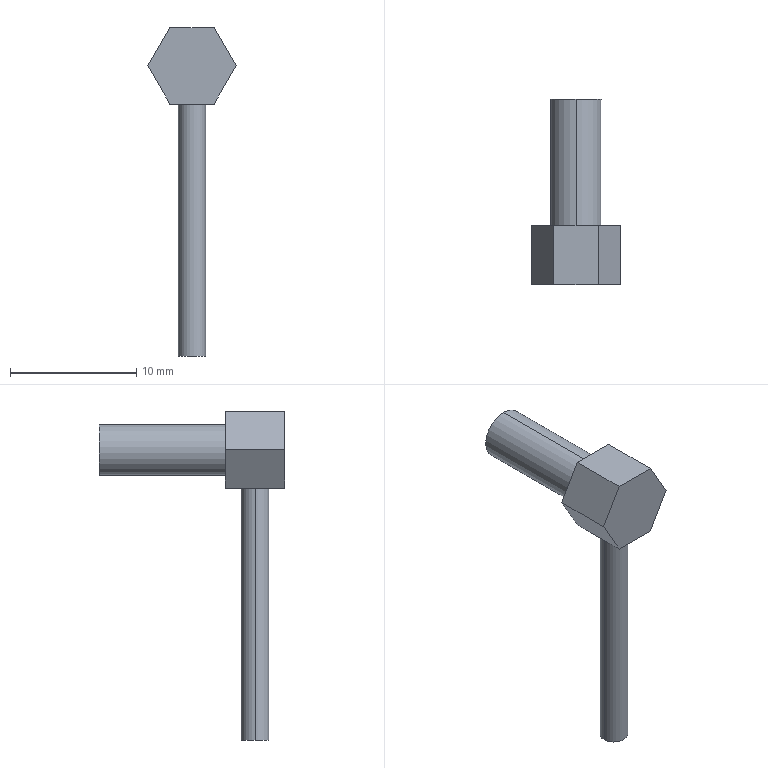Part | STEP file | E32-T11N 2M(欧姆龙280mm) | 1 solid | 17 faces | box 7 x 14.7 x 26.062 mm | volume 350.96 mm3 | plane 11 | cylinder 6 | commonest cylinder face diameters 2 x2 2.2 x2 4 x2
STEP:
#1=CARTESIAN_POINT('',(0.,0.,0.));
#2=DIRECTION('',(0.,0.,1.));
#3=DIRECTION('',(1.,0.,0.));
#4=AXIS2_PLACEMENT_3D('',#1,#2,#3);
#5=CARTESIAN_POINT('',(-1.1,-7.35,-23.031));
#6=VERTEX_POINT('',#5);
#7=CARTESIAN_POINT('',(1.1,-7.35,-23.031));
#8=VERTEX_POINT('',#7);
#9=CARTESIAN_POINT('',(0.,-7.35,-23.031));
#10=DIRECTION('',(0.,0.,-1.));
#11=DIRECTION('',(-1.,0.,0.));
#12=AXIS2_PLACEMENT_3D('',#9,#10,#11);
#13=CIRCLE('',#12,1.1);
#14=CARTESIAN_POINT('',(0.,-7.35,-23.031));
#15=DIRECTION('',(0.,0.,1.));
#16=DIRECTION('',(1.,0.,0.));
#17=AXIS2_PLACEMENT_3D('',#14,#15,#16);
#18=CYLINDRICAL_SURFACE('',#17,1.1);
#19=CARTESIAN_POINT('',(3.142,0.));
#20=DIRECTION('',(-1.,0.));
#21=VECTOR('',#20,1.);
#22=LINE('',#19,#21);
#23=(GEOMETRIC_REPRESENTATION_CONTEXT(2)PARAMETRIC_REPRESENTATION_CONTEXT()REPRESENTATION_CONTEXT('',''));
#24=DEFINITIONAL_REPRESENTATION('',(#22),#23);
#25=PCURVE('',#18,#24);
#26=CARTESIAN_POINT('',(0.,-7.35,-23.031));
#27=DIRECTION('',(0.,0.,-1.));
#28=DIRECTION('',(-1.,0.,0.));
#29=AXIS2_PLACEMENT_3D('',#26,#27,#28);
#30=PLANE('',#29);
#31=CARTESIAN_POINT('',(0.,0.));
#32=DIRECTION('',(1.,0.));
#33=AXIS2_PLACEMENT_2D('',#31,#32);
#34=CIRCLE('',#33,1.1);
#35=(GEOMETRIC_REPRESENTATION_CONTEXT(2)PARAMETRIC_REPRESENTATION_CONTEXT()REPRESENTATION_CONTEXT('',''));
#36=DEFINITIONAL_REPRESENTATION('',(#34),#35);
#37=PCURVE('',#30,#36);
#38=SURFACE_CURVE('',#13,(#25,#37),.PCURVE_S1.);
#39=EDGE_CURVE('',#6,#8,#38,.T.);
#40=ORIENTED_EDGE('',*,*,#39,.F.);
#41=CARTESIAN_POINT('',(-1.1,-7.35,-3.031));
#42=VERTEX_POINT('',#41);
#43=CARTESIAN_POINT('',(-1.1,-7.35,-23.031));
#44=DIRECTION('',(0.,0.,1.));
#45=VECTOR('',#44,1.);
#46=LINE('',#43,#45);
#47=CARTESIAN_POINT('',(3.142,0.));
#48=DIRECTION('',(0.,1.));
#49=VECTOR('',#48,1.);
#50=LINE('',#47,#49);
#51=(GEOMETRIC_REPRESENTATION_CONTEXT(2)PARAMETRIC_REPRESENTATION_CONTEXT()REPRESENTATION_CONTEXT('',''));
#52=DEFINITIONAL_REPRESENTATION('',(#50),#51);
#53=PCURVE('',#18,#52);
#54=CARTESIAN_POINT('',(0.,-7.35,-23.031));
#55=DIRECTION('',(0.,0.,1.));
#56=DIRECTION('',(1.,0.,0.));
#57=AXIS2_PLACEMENT_3D('',#54,#55,#56);
#58=CYLINDRICAL_SURFACE('',#57,1.1);
#59=CARTESIAN_POINT('',(3.142,0.));
#60=DIRECTION('',(0.,1.));
#61=VECTOR('',#60,1.);
#62=LINE('',#59,#61);
#63=(GEOMETRIC_REPRESENTATION_CONTEXT(2)PARAMETRIC_REPRESENTATION_CONTEXT()REPRESENTATION_CONTEXT('',''));
#64=DEFINITIONAL_REPRESENTATION('',(#62),#63);
#65=PCURVE('',#58,#64);
#66=SURFACE_CURVE('',#46,(#53,#65),.PCURVE_S1.);
#67=EDGE_CURVE('',#6,#42,#66,.T.);
#68=ORIENTED_EDGE('',*,*,#67,.T.);
#69=CARTESIAN_POINT('',(1.1,-7.35,-3.031));
#70=VERTEX_POINT('',#69);
#71=CARTESIAN_POINT('',(0.,-7.35,-3.031));
#72=DIRECTION('',(0.,0.,-1.));
#73=DIRECTION('',(-1.,0.,0.));
#74=AXIS2_PLACEMENT_3D('',#71,#72,#73);
#75=CIRCLE('',#74,1.1);
#76=CARTESIAN_POINT('',(3.142,20.));
#77=DIRECTION('',(-1.,0.));
#78=VECTOR('',#77,1.);
#79=LINE('',#76,#78);
#80=(GEOMETRIC_REPRESENTATION_CONTEXT(2)PARAMETRIC_REPRESENTATION_CONTEXT()REPRESENTATION_CONTEXT('',''));
#81=DEFINITIONAL_REPRESENTATION('',(#79),#80);
#82=PCURVE('',#18,#81);
#83=CARTESIAN_POINT('',(-1.75,-9.7,-3.031));
#84=DIRECTION('',(0.,0.,1.));
#85=DIRECTION('',(1.,0.,0.));
#86=AXIS2_PLACEMENT_3D('',#83,#84,#85);
#87=PLANE('',#86);
#88=CARTESIAN_POINT('',(0.65,2.35));
#89=CARTESIAN_POINT('',(0.65,4.255));
#90=CARTESIAN_POINT('',(2.3,3.303));
#91=CARTESIAN_POINT('',(3.95,2.35));
#92=CARTESIAN_POINT('',(2.3,1.397));
#93=CARTESIAN_POINT('',(0.65,0.4447));
#94=CARTESIAN_POINT('',(0.65,2.35));
#95=(BOUNDED_CURVE()B_SPLINE_CURVE(2,(#88,#89,#90,#91,#92,#93,#94),.UNSPECIFIED.,.T.,.F.)B_SPLINE_CURVE_WITH_KNOTS((1,2,2,2,2,1),(-2.094,0.,2.094,4.189,6.283,8.378),.UNSPECIFIED.)CURVE()GEOMETRIC_REPRESENTATION_ITEM()RATIONAL_B_SPLINE_CURVE((1.,0.5,1.,0.5,1.,0.5,1.))REPRESENTATION_ITEM(''));
#96=(GEOMETRIC_REPRESENTATION_CONTEXT(2)PARAMETRIC_REPRESENTATION_CONTEXT()REPRESENTATION_CONTEXT('',''));
#97=DEFINITIONAL_REPRESENTATION('',(#95),#96);
#98=PCURVE('',#87,#97);
#99=SURFACE_CURVE('',#75,(#82,#98),.PCURVE_S1.);
#100=EDGE_CURVE('',#42,#70,#99,.T.);
#101=ORIENTED_EDGE('',*,*,#100,.T.);
#102=CARTESIAN_POINT('',(1.1,-7.35,-23.031));
#103=DIRECTION('',(0.,0.,1.));
#104=VECTOR('',#103,1.);
#105=LINE('',#102,#104);
#106=CARTESIAN_POINT('',(0.,0.));
#107=DIRECTION('',(0.,1.));
#108=VECTOR('',#107,1.);
#109=LINE('',#106,#108);
#110=(GEOMETRIC_REPRESENTATION_CONTEXT(2)PARAMETRIC_REPRESENTATION_CONTEXT()REPRESENTATION_CONTEXT('',''));
#111=DEFINITIONAL_REPRESENTATION('',(#109),#110);
#112=PCURVE('',#18,#111);
#113=CARTESIAN_POINT('',(6.283,0.));
#114=DIRECTION('',(0.,1.));
#115=VECTOR('',#114,1.);
#116=LINE('',#113,#115);
#117=(GEOMETRIC_REPRESENTATION_CONTEXT(2)PARAMETRIC_REPRESENTATION_CONTEXT()REPRESENTATION_CONTEXT('',''));
#118=DEFINITIONAL_REPRESENTATION('',(#116),#117);
#119=PCURVE('',#58,#118);
#120=SURFACE_CURVE('',#105,(#112,#119),.PCURVE_S1.);
#121=EDGE_CURVE('',#8,#70,#120,.T.);
#122=ORIENTED_EDGE('',*,*,#121,.F.);
#123=EDGE_LOOP('',(#40,#68,#101,#122));
#124=FACE_BOUND('',#123,.T.);
#125=ADVANCED_FACE('',(#124),#18,.T.);
#126=CARTESIAN_POINT('',(0.,4.9,1.));
#127=VERTEX_POINT('',#126);
#128=CARTESIAN_POINT('',(0.,5.,1.));
#129=VERTEX_POINT('',#128);
#130=CARTESIAN_POINT('',(0.,4.9,1.));
#131=DIRECTION('',(0.,1.,0.));
#132=VECTOR('',#131,1.);
#133=LINE('',#130,#132);
#134=CARTESIAN_POINT('',(0.,4.9,0.));
#135=DIRECTION('',(0.,1.,0.));
#136=DIRECTION('',(0.,0.,1.));
#137=AXIS2_PLACEMENT_3D('',#134,#135,#136);
#138=CYLINDRICAL_SURFACE('',#137,1.);
#139=CARTESIAN_POINT('',(6.283,0.));
#140=DIRECTION('',(0.,1.));
#141=VECTOR('',#140,1.);
#142=LINE('',#139,#141);
#143=(GEOMETRIC_REPRESENTATION_CONTEXT(2)PARAMETRIC_REPRESENTATION_CONTEXT()REPRESENTATION_CONTEXT('',''));
#144=DEFINITIONAL_REPRESENTATION('',(#142),#143);
#145=PCURVE('',#138,#144);
#146=CARTESIAN_POINT('',(0.,4.9,0.));
#147=DIRECTION('',(0.,1.,0.));
#148=DIRECTION('',(0.,0.,1.));
#149=AXIS2_PLACEMENT_3D('',#146,#147,#148);
#150=CYLINDRICAL_SURFACE('',#149,1.);
#151=CARTESIAN_POINT('',(0.,0.));
#152=DIRECTION('',(0.,1.));
#153=VECTOR('',#152,1.);
#154=LINE('',#151,#153);
#155=(GEOMETRIC_REPRESENTATION_CONTEXT(2)PARAMETRIC_REPRESENTATION_CONTEXT()REPRESENTATION_CONTEXT('',''));
#156=DEFINITIONAL_REPRESENTATION('',(#154),#155);
#157=PCURVE('',#150,#156);
#158=SURFACE_CURVE('',#133,(#145,#157),.PCURVE_S1.);
#159=EDGE_CURVE('',#127,#129,#158,.T.);
#160=ORIENTED_EDGE('',*,*,#159,.T.);
#161=CARTESIAN_POINT('',(0.,5.,-1.));
#162=VERTEX_POINT('',#161);
#163=CARTESIAN_POINT('',(0.,5.,0.));
#164=DIRECTION('',(0.,1.,0.));
#165=DIRECTION('',(0.,0.,1.));
#166=AXIS2_PLACEMENT_3D('',#163,#164,#165);
#167=CIRCLE('',#166,1.);
#168=CARTESIAN_POINT('',(0.,0.1));
#169=DIRECTION('',(1.,0.));
#170=VECTOR('',#169,1.);
#171=LINE('',#168,#170);
#172=(GEOMETRIC_REPRESENTATION_CONTEXT(2)PARAMETRIC_REPRESENTATION_CONTEXT()REPRESENTATION_CONTEXT('',''));
#173=DEFINITIONAL_REPRESENTATION('',(#171),#172);
#174=PCURVE('',#138,#173);
#175=CARTESIAN_POINT('',(0.,5.,0.));
#176=DIRECTION('',(0.,1.,0.));
#177=DIRECTION('',(0.,0.,1.));
#178=AXIS2_PLACEMENT_3D('',#175,#176,#177);
#179=PLANE('',#178);
#180=CARTESIAN_POINT('',(0.,0.));
#181=DIRECTION('',(1.,0.));
#182=AXIS2_PLACEMENT_2D('',#180,#181);
#183=CIRCLE('',#182,1.);
#184=(GEOMETRIC_REPRESENTATION_CONTEXT(2)PARAMETRIC_REPRESENTATION_CONTEXT()REPRESENTATION_CONTEXT('',''));
#185=DEFINITIONAL_REPRESENTATION('',(#183),#184);
#186=PCURVE('',#179,#185);
#187=SURFACE_CURVE('',#167,(#174,#186),.PCURVE_S1.);
#188=EDGE_CURVE('',#162,#129,#187,.T.);
#189=ORIENTED_EDGE('',*,*,#188,.F.);
#190=CARTESIAN_POINT('',(0.,4.9,-1.));
#191=VERTEX_POINT('',#190);
#192=CARTESIAN_POINT('',(0.,4.9,-1.));
#193=DIRECTION('',(0.,1.,0.));
#194=VECTOR('',#193,1.);
#195=LINE('',#192,#194);
#196=CARTESIAN_POINT('',(3.142,0.));
#197=DIRECTION('',(0.,1.));
#198=VECTOR('',#197,1.);
#199=LINE('',#196,#198);
#200=(GEOMETRIC_REPRESENTATION_CONTEXT(2)PARAMETRIC_REPRESENTATION_CONTEXT()REPRESENTATION_CONTEXT('',''));
#201=DEFINITIONAL_REPRESENTATION('',(#199),#200);
#202=PCURVE('',#138,#201);
#203=CARTESIAN_POINT('',(3.142,0.));
#204=DIRECTION('',(0.,1.));
#205=VECTOR('',#204,1.);
#206=LINE('',#203,#205);
#207=(GEOMETRIC_REPRESENTATION_CONTEXT(2)PARAMETRIC_REPRESENTATION_CONTEXT()REPRESENTATION_CONTEXT('',''));
#208=DEFINITIONAL_REPRESENTATION('',(#206),#207);
#209=PCURVE('',#150,#208);
#210=SURFACE_CURVE('',#195,(#202,#209),.PCURVE_S1.);
#211=EDGE_CURVE('',#191,#162,#210,.T.);
#212=ORIENTED_EDGE('',*,*,#211,.F.);
#213=CARTESIAN_POINT('',(0.,4.9,0.));
#214=DIRECTION('',(0.,1.,0.));
#215=DIRECTION('',(0.,0.,1.));
#216=AXIS2_PLACEMENT_3D('',#213,#214,#215);
#217=CIRCLE('',#216,1.);
#218=CARTESIAN_POINT('',(0.,0.));
#219=DIRECTION('',(1.,0.));
#220=VECTOR('',#219,1.);
#221=LINE('',#218,#220);
#222=(GEOMETRIC_REPRESENTATION_CONTEXT(2)PARAMETRIC_REPRESENTATION_CONTEXT()REPRESENTATION_CONTEXT('',''));
#223=DEFINITIONAL_REPRESENTATION('',(#221),#222);
#224=PCURVE('',#138,#223);
#225=CARTESIAN_POINT('',(0.,4.9,0.));
#226=DIRECTION('',(0.,1.,0.));
#227=DIRECTION('',(0.,0.,1.));
#228=AXIS2_PLACEMENT_3D('',#225,#226,#227);
#229=PLANE('',#228);
#230=CARTESIAN_POINT('',(0.,0.));
#231=DIRECTION('',(1.,0.));
#232=AXIS2_PLACEMENT_2D('',#230,#231);
#233=CIRCLE('',#232,1.);
#234=(GEOMETRIC_REPRESENTATION_CONTEXT(2)PARAMETRIC_REPRESENTATION_CONTEXT()REPRESENTATION_CONTEXT('',''));
#235=DEFINITIONAL_REPRESENTATION('',(#233),#234);
#236=PCURVE('',#229,#235);
#237=SURFACE_CURVE('',#217,(#224,#236),.PCURVE_S1.);
#238=EDGE_CURVE('',#191,#127,#237,.T.);
#239=ORIENTED_EDGE('',*,*,#238,.T.);
#240=EDGE_LOOP('',(#160,#189,#212,#239));
#241=FACE_BOUND('',#240,.F.);
#242=ADVANCED_FACE('',(#241),#138,.F.);
#243=CARTESIAN_POINT('',(0.,5.,2.));
#244=VERTEX_POINT('',#243);
#245=CARTESIAN_POINT('',(0.,5.,-2.));
#246=VERTEX_POINT('',#245);
#247=CARTESIAN_POINT('',(0.,5.,0.));
#248=DIRECTION('',(0.,1.,0.));
#249=DIRECTION('',(0.,0.,1.));
#250=AXIS2_PLACEMENT_3D('',#247,#248,#249);
#251=CIRCLE('',#250,2.);
#252=CARTESIAN_POINT('',(0.,5.,0.));
#253=DIRECTION('',(0.,-1.,0.));
#254=DIRECTION('',(0.,0.,-1.));
#255=AXIS2_PLACEMENT_3D('',#252,#253,#254);
#256=CYLINDRICAL_SURFACE('',#255,2.);
#257=CARTESIAN_POINT('',(3.142,0.));
#258=DIRECTION('',(-1.,0.));
#259=VECTOR('',#258,1.);
#260=LINE('',#257,#259);
#261=(GEOMETRIC_REPRESENTATION_CONTEXT(2)PARAMETRIC_REPRESENTATION_CONTEXT()REPRESENTATION_CONTEXT('',''));
#262=DEFINITIONAL_REPRESENTATION('',(#260),#261);
#263=PCURVE('',#256,#262);
#264=CARTESIAN_POINT('',(0.,0.));
#265=DIRECTION('',(1.,0.));
#266=AXIS2_PLACEMENT_2D('',#264,#265);
#267=CIRCLE('',#266,2.);
#268=(GEOMETRIC_REPRESENTATION_CONTEXT(2)PARAMETRIC_REPRESENTATION_CONTEXT()REPRESENTATION_CONTEXT('',''));
#269=DEFINITIONAL_REPRESENTATION('',(#267),#268);
#270=PCURVE('',#179,#269);
#271=SURFACE_CURVE('',#251,(#263,#270),.PCURVE_S1.);
#272=EDGE_CURVE('',#244,#246,#271,.T.);
#273=ORIENTED_EDGE('',*,*,#272,.F.);
#274=CARTESIAN_POINT('',(0.,-5.,2.));
#275=VERTEX_POINT('',#274);
#276=CARTESIAN_POINT('',(0.,5.,2.));
#277=DIRECTION('',(0.,-1.,0.));
#278=VECTOR('',#277,1.);
#279=LINE('',#276,#278);
#280=CARTESIAN_POINT('',(3.142,0.));
#281=DIRECTION('',(0.,1.));
#282=VECTOR('',#281,1.);
#283=LINE('',#280,#282);
#284=(GEOMETRIC_REPRESENTATION_CONTEXT(2)PARAMETRIC_REPRESENTATION_CONTEXT()REPRESENTATION_CONTEXT('',''));
#285=DEFINITIONAL_REPRESENTATION('',(#283),#284);
#286=PCURVE('',#256,#285);
#287=CARTESIAN_POINT('',(0.,5.,0.));
#288=DIRECTION('',(0.,-1.,0.));
#289=DIRECTION('',(0.,0.,-1.));
#290=AXIS2_PLACEMENT_3D('',#287,#288,#289);
#291=CYLINDRICAL_SURFACE('',#290,2.);
#292=CARTESIAN_POINT('',(3.142,0.));
#293=DIRECTION('',(0.,1.));
#294=VECTOR('',#293,1.);
#295=LINE('',#292,#294);
#296=(GEOMETRIC_REPRESENTATION_CONTEXT(2)PARAMETRIC_REPRESENTATION_CONTEXT()REPRESENTATION_CONTEXT('',''));
#297=DEFINITIONAL_REPRESENTATION('',(#295),#296);
#298=PCURVE('',#291,#297);
#299=SURFACE_CURVE('',#279,(#286,#298),.PCURVE_S1.);
#300=EDGE_CURVE('',#244,#275,#299,.T.);
#301=ORIENTED_EDGE('',*,*,#300,.T.);
#302=CARTESIAN_POINT('',(0.,-5.,-2.));
#303=VERTEX_POINT('',#302);
#304=CARTESIAN_POINT('',(0.,-5.,0.));
#305=DIRECTION('',(0.,1.,0.));
#306=DIRECTION('',(0.,0.,1.));
#307=AXIS2_PLACEMENT_3D('',#304,#305,#306);
#308=CIRCLE('',#307,2.);
#309=CARTESIAN_POINT('',(3.142,10.));
#310=DIRECTION('',(-1.,0.));
#311=VECTOR('',#310,1.);
#312=LINE('',#309,#311);
#313=(GEOMETRIC_REPRESENTATION_CONTEXT(2)PARAMETRIC_REPRESENTATION_CONTEXT()REPRESENTATION_CONTEXT('',''));
#314=DEFINITIONAL_REPRESENTATION('',(#312),#313);
#315=PCURVE('',#256,#314);
#316=CARTESIAN_POINT('',(0.,-5.,0.));
#317=DIRECTION('',(0.,-1.,0.));
#318=DIRECTION('',(0.,0.,-1.));
#319=AXIS2_PLACEMENT_3D('',#316,#317,#318);
#320=PLANE('',#319);
#321=CARTESIAN_POINT('',(-2.,0.));
#322=CARTESIAN_POINT('',(-2.,3.464));
#323=CARTESIAN_POINT('',(1.,1.732));
#324=CARTESIAN_POINT('',(4.,0.));
#325=CARTESIAN_POINT('',(1.,-1.732));
#326=CARTESIAN_POINT('',(-2.,-3.464));
#327=CARTESIAN_POINT('',(-2.,0.));
#328=(BOUNDED_CURVE()B_SPLINE_CURVE(2,(#321,#322,#323,#324,#325,#326,#327),.UNSPECIFIED.,.T.,.F.)B_SPLINE_CURVE_WITH_KNOTS((1,2,2,2,2,1),(-2.094,0.,2.094,4.189,6.283,8.378),.UNSPECIFIED.)CURVE()GEOMETRIC_REPRESENTATION_ITEM()RATIONAL_B_SPLINE_CURVE((1.,0.5,1.,0.5,1.,0.5,1.))REPRESENTATION_ITEM(''));
#329=(GEOMETRIC_REPRESENTATION_CONTEXT(2)PARAMETRIC_REPRESENTATION_CONTEXT()REPRESENTATION_CONTEXT('',''));
#330=DEFINITIONAL_REPRESENTATION('',(#328),#329);
#331=PCURVE('',#320,#330);
#332=SURFACE_CURVE('',#308,(#315,#331),.PCURVE_S1.);
#333=EDGE_CURVE('',#275,#303,#332,.T.);
#334=ORIENTED_EDGE('',*,*,#333,.T.);
#335=CARTESIAN_POINT('',(0.,5.,-2.));
#336=DIRECTION('',(0.,-1.,0.));
#337=VECTOR('',#336,1.);
#338=LINE('',#335,#337);
#339=CARTESIAN_POINT('',(0.,0.));
#340=DIRECTION('',(0.,1.));
#341=VECTOR('',#340,1.);
#342=LINE('',#339,#341);
#343=(GEOMETRIC_REPRESENTATION_CONTEXT(2)PARAMETRIC_REPRESENTATION_CONTEXT()REPRESENTATION_CONTEXT('',''));
#344=DEFINITIONAL_REPRESENTATION('',(#342),#343);
#345=PCURVE('',#256,#344);
#346=CARTESIAN_POINT('',(6.283,0.));
#347=DIRECTION('',(0.,1.));
#348=VECTOR('',#347,1.);
#349=LINE('',#346,#348);
#350=(GEOMETRIC_REPRESENTATION_CONTEXT(2)PARAMETRIC_REPRESENTATION_CONTEXT()REPRESENTATION_CONTEXT('',''));
#351=DEFINITIONAL_REPRESENTATION('',(#349),#350);
#352=PCURVE('',#291,#351);
#353=SURFACE_CURVE('',#338,(#345,#352),.PCURVE_S1.);
#354=EDGE_CURVE('',#246,#303,#353,.T.);
#355=ORIENTED_EDGE('',*,*,#354,.F.);
#356=EDGE_LOOP('',(#273,#301,#334,#355));
#357=FACE_BOUND('',#356,.T.);
#358=ADVANCED_FACE('',(#357),#256,.T.);
#359=ORIENTED_EDGE('',*,*,#300,.F.);
#360=CARTESIAN_POINT('',(0.,5.,0.));
#361=DIRECTION('',(0.,1.,0.));
#362=DIRECTION('',(0.,0.,1.));
#363=AXIS2_PLACEMENT_3D('',#360,#361,#362);
#364=CIRCLE('',#363,2.);
#365=CARTESIAN_POINT('',(9.425,0.));
#366=DIRECTION('',(-1.,0.));
#367=VECTOR('',#366,1.);
#368=LINE('',#365,#367);
#369=(GEOMETRIC_REPRESENTATION_CONTEXT(2)PARAMETRIC_REPRESENTATION_CONTEXT()REPRESENTATION_CONTEXT('',''));
#370=DEFINITIONAL_REPRESENTATION('',(#368),#369);
#371=PCURVE('',#291,#370);
#372=CARTESIAN_POINT('',(0.,0.));
#373=DIRECTION('',(1.,0.));
#374=AXIS2_PLACEMENT_2D('',#372,#373);
#375=CIRCLE('',#374,2.);
#376=(GEOMETRIC_REPRESENTATION_CONTEXT(2)PARAMETRIC_REPRESENTATION_CONTEXT()REPRESENTATION_CONTEXT('',''));
#377=DEFINITIONAL_REPRESENTATION('',(#375),#376);
#378=PCURVE('',#179,#377);
#379=SURFACE_CURVE('',#364,(#371,#378),.PCURVE_S1.);
#380=EDGE_CURVE('',#246,#244,#379,.T.);
#381=ORIENTED_EDGE('',*,*,#380,.F.);
#382=ORIENTED_EDGE('',*,*,#354,.T.);
#383=CARTESIAN_POINT('',(0.,-5.,0.));
#384=DIRECTION('',(0.,1.,0.));
#385=DIRECTION('',(0.,0.,1.));
#386=AXIS2_PLACEMENT_3D('',#383,#384,#385);
#387=CIRCLE('',#386,2.);
#388=CARTESIAN_POINT('',(9.425,10.));
#389=DIRECTION('',(-1.,0.));
#390=VECTOR('',#389,1.);
#391=LINE('',#388,#390);
#392=(GEOMETRIC_REPRESENTATION_CONTEXT(2)PARAMETRIC_REPRESENTATION_CONTEXT()REPRESENTATION_CONTEXT('',''));
#393=DEFINITIONAL_REPRESENTATION('',(#391),#392);
#394=PCURVE('',#291,#393);
#395=CARTESIAN_POINT('',(-2.,0.));
#396=CARTESIAN_POINT('',(-2.,3.464));
#397=CARTESIAN_POINT('',(1.,1.732));
#398=CARTESIAN_POINT('',(4.,0.));
#399=CARTESIAN_POINT('',(1.,-1.732));
#400=CARTESIAN_POINT('',(-2.,-3.464));
#401=CARTESIAN_POINT('',(-2.,0.));
#402=(BOUNDED_CURVE()B_SPLINE_CURVE(2,(#395,#396,#397,#398,#399,#400,#401),.UNSPECIFIED.,.T.,.F.)B_SPLINE_CURVE_WITH_KNOTS((1,2,2,2,2,1),(-2.094,0.,2.094,4.189,6.283,8.378),.UNSPECIFIED.)CURVE()GEOMETRIC_REPRESENTATION_ITEM()RATIONAL_B_SPLINE_CURVE((1.,0.5,1.,0.5,1.,0.5,1.))REPRESENTATION_ITEM(''));
#403=(GEOMETRIC_REPRESENTATION_CONTEXT(2)PARAMETRIC_REPRESENTATION_CONTEXT()REPRESENTATION_CONTEXT('',''));
#404=DEFINITIONAL_REPRESENTATION('',(#402),#403);
#405=PCURVE('',#320,#404);
#406=SURFACE_CURVE('',#387,(#394,#405),.PCURVE_S1.);
#407=EDGE_CURVE('',#303,#275,#406,.T.);
#408=ORIENTED_EDGE('',*,*,#407,.T.);
#409=EDGE_LOOP('',(#359,#381,#382,#408));
#410=FACE_BOUND('',#409,.T.);
#411=ADVANCED_FACE('',(#410),#291,.T.);
#412=CARTESIAN_POINT('',(0.,5.,0.));
#413=DIRECTION('',(0.,1.,0.));
#414=DIRECTION('',(0.,0.,1.));
#415=AXIS2_PLACEMENT_3D('',#412,#413,#414);
#416=CIRCLE('',#415,1.);
#417=CARTESIAN_POINT('',(0.,0.));
#418=DIRECTION('',(1.,0.));
#419=AXIS2_PLACEMENT_2D('',#417,#418);
#420=CIRCLE('',#419,1.);
#421=(GEOMETRIC_REPRESENTATION_CONTEXT(2)PARAMETRIC_REPRESENTATION_CONTEXT()REPRESENTATION_CONTEXT('',''));
#422=DEFINITIONAL_REPRESENTATION('',(#420),#421);
#423=PCURVE('',#179,#422);
#424=CARTESIAN_POINT('',(0.,0.1));
#425=DIRECTION('',(1.,0.));
#426=VECTOR('',#425,1.);
#427=LINE('',#424,#426);
#428=(GEOMETRIC_REPRESENTATION_CONTEXT(2)PARAMETRIC_REPRESENTATION_CONTEXT()REPRESENTATION_CONTEXT('',''));
#429=DEFINITIONAL_REPRESENTATION('',(#427),#428);
#430=PCURVE('',#150,#429);
#431=SURFACE_CURVE('',#416,(#423,#430),.PCURVE_S1.);
#432=EDGE_CURVE('',#129,#162,#431,.T.);
#433=ORIENTED_EDGE('',*,*,#432,.F.);
#434=ORIENTED_EDGE('',*,*,#188,.F.);
#435=EDGE_LOOP('',(#433,#434));
#436=FACE_BOUND('',#435,.T.);
#437=ORIENTED_EDGE('',*,*,#380,.T.);
#438=ORIENTED_EDGE('',*,*,#272,.T.);
#439=EDGE_LOOP('',(#437,#438));
#440=FACE_BOUND('',#439,.T.);
#441=ADVANCED_FACE('',(#436,#440),#179,.T.);
#442=ORIENTED_EDGE('',*,*,#432,.F.);
#443=ORIENTED_EDGE('',*,*,#159,.F.);
#444=CARTESIAN_POINT('',(0.,4.9,0.));
#445=DIRECTION('',(0.,1.,0.));
#446=DIRECTION('',(0.,0.,1.));
#447=AXIS2_PLACEMENT_3D('',#444,#445,#446);
#448=CIRCLE('',#447,1.);
#449=CARTESIAN_POINT('',(0.,0.));
#450=DIRECTION('',(1.,0.));
#451=VECTOR('',#450,1.);
#452=LINE('',#449,#451);
#453=(GEOMETRIC_REPRESENTATION_CONTEXT(2)PARAMETRIC_REPRESENTATION_CONTEXT()REPRESENTATION_CONTEXT('',''));
#454=DEFINITIONAL_REPRESENTATION('',(#452),#453);
#455=PCURVE('',#150,#454);
#456=CARTESIAN_POINT('',(0.,0.));
#457=DIRECTION('',(1.,0.));
#458=AXIS2_PLACEMENT_2D('',#456,#457);
#459=CIRCLE('',#458,1.);
#460=(GEOMETRIC_REPRESENTATION_CONTEXT(2)PARAMETRIC_REPRESENTATION_CONTEXT()REPRESENTATION_CONTEXT('',''));
#461=DEFINITIONAL_REPRESENTATION('',(#459),#460);
#462=PCURVE('',#229,#461);
#463=SURFACE_CURVE('',#448,(#455,#462),.PCURVE_S1.);
#464=EDGE_CURVE('',#127,#191,#463,.T.);
#465=ORIENTED_EDGE('',*,*,#464,.T.);
#466=ORIENTED_EDGE('',*,*,#211,.T.);
#467=EDGE_LOOP('',(#442,#443,#465,#466));
#468=FACE_BOUND('',#467,.F.);
#469=ADVANCED_FACE('',(#468),#150,.F.);
#470=ORIENTED_EDGE('',*,*,#464,.T.);
#471=ORIENTED_EDGE('',*,*,#238,.T.);
#472=EDGE_LOOP('',(#470,#471));
#473=FACE_BOUND('',#472,.T.);
#474=ADVANCED_FACE('',(#473),#229,.T.);
#475=CARTESIAN_POINT('',(1.75,-5.,3.031));
#476=VERTEX_POINT('',#475);
#477=CARTESIAN_POINT('',(-1.75,-5.,3.031));
#478=VERTEX_POINT('',#477);
#479=CARTESIAN_POINT('',(1.75,-5.,3.031));
#480=DIRECTION('',(-1.,0.,0.));
#481=VECTOR('',#480,1.);
#482=LINE('',#479,#481);
#483=CARTESIAN_POINT('',(1.75,-9.7,3.031));
#484=DIRECTION('',(0.,0.,-1.));
#485=DIRECTION('',(-1.,0.,0.));
#486=AXIS2_PLACEMENT_3D('',#483,#484,#485);
#487=PLANE('',#486);
#488=CARTESIAN_POINT('',(0.,4.7));
#489=DIRECTION('',(1.,0.));
#490=VECTOR('',#489,1.);
#491=LINE('',#488,#490);
#492=(GEOMETRIC_REPRESENTATION_CONTEXT(2)PARAMETRIC_REPRESENTATION_CONTEXT()REPRESENTATION_CONTEXT('',''));
#493=DEFINITIONAL_REPRESENTATION('',(#491),#492);
#494=PCURVE('',#487,#493);
#495=CARTESIAN_POINT('',(-3.031,1.75));
#496=DIRECTION('',(0.,-1.));
#497=VECTOR('',#496,1.);
#498=LINE('',#495,#497);
#499=(GEOMETRIC_REPRESENTATION_CONTEXT(2)PARAMETRIC_REPRESENTATION_CONTEXT()REPRESENTATION_CONTEXT('',''));
#500=DEFINITIONAL_REPRESENTATION('',(#498),#499);
#501=PCURVE('',#320,#500);
#502=SURFACE_CURVE('',#482,(#494,#501),.PCURVE_S1.);
#503=EDGE_CURVE('',#476,#478,#502,.T.);
#504=ORIENTED_EDGE('',*,*,#503,.T.);
#505=CARTESIAN_POINT('',(-1.75,-9.7,3.031));
#506=VERTEX_POINT('',#505);
#507=CARTESIAN_POINT('',(-1.75,-9.7,3.031));
#508=DIRECTION('',(0.,1.,0.));
#509=VECTOR('',#508,1.);
#510=LINE('',#507,#509);
#511=CARTESIAN_POINT('',(3.5,0.));
#512=DIRECTION('',(0.,1.));
#513=VECTOR('',#512,1.);
#514=LINE('',#511,#513);
#515=(GEOMETRIC_REPRESENTATION_CONTEXT(2)PARAMETRIC_REPRESENTATION_CONTEXT()REPRESENTATION_CONTEXT('',''));
#516=DEFINITIONAL_REPRESENTATION('',(#514),#515);
#517=PCURVE('',#487,#516);
#518=CARTESIAN_POINT('',(-1.75,-9.7,3.031));
#519=DIRECTION('',(0.866,0.,-0.5));
#520=DIRECTION('',(-0.5,0.,-0.866));
#521=AXIS2_PLACEMENT_3D('',#518,#519,#520);
#522=PLANE('',#521);
#523=CARTESIAN_POINT('',(0.,0.));
#524=DIRECTION('',(0.,1.));
#525=VECTOR('',#524,1.);
#526=LINE('',#523,#525);
#527=(GEOMETRIC_REPRESENTATION_CONTEXT(2)PARAMETRIC_REPRESENTATION_CONTEXT()REPRESENTATION_CONTEXT('',''));
#528=DEFINITIONAL_REPRESENTATION('',(#526),#527);
#529=PCURVE('',#522,#528);
#530=SURFACE_CURVE('',#510,(#517,#529),.PCURVE_S1.);
#531=EDGE_CURVE('',#506,#478,#530,.T.);
#532=ORIENTED_EDGE('',*,*,#531,.F.);
#533=CARTESIAN_POINT('',(1.75,-9.7,3.031));
#534=VERTEX_POINT('',#533);
#535=CARTESIAN_POINT('',(1.75,-9.7,3.031));
#536=DIRECTION('',(-1.,0.,0.));
#537=VECTOR('',#536,1.);
#538=LINE('',#535,#537);
#539=CARTESIAN_POINT('',(0.,0.));
#540=DIRECTION('',(1.,0.));
#541=VECTOR('',#540,1.);
#542=LINE('',#539,#541);
#543=(GEOMETRIC_REPRESENTATION_CONTEXT(2)PARAMETRIC_REPRESENTATION_CONTEXT()REPRESENTATION_CONTEXT('',''));
#544=DEFINITIONAL_REPRESENTATION('',(#542),#543);
#545=PCURVE('',#487,#544);
#546=CARTESIAN_POINT('',(0.,-9.7,0.));
#547=DIRECTION('',(0.,-1.,0.));
#548=DIRECTION('',(0.,0.,-1.));
#549=AXIS2_PLACEMENT_3D('',#546,#547,#548);
#550=PLANE('',#549);
#551=CARTESIAN_POINT('',(-3.031,1.75));
#552=DIRECTION('',(0.,-1.));
#553=VECTOR('',#552,1.);
#554=LINE('',#551,#553);
#555=(GEOMETRIC_REPRESENTATION_CONTEXT(2)PARAMETRIC_REPRESENTATION_CONTEXT()REPRESENTATION_CONTEXT('',''));
#556=DEFINITIONAL_REPRESENTATION('',(#554),#555);
#557=PCURVE('',#550,#556);
#558=SURFACE_CURVE('',#538,(#545,#557),.PCURVE_S1.);
#559=EDGE_CURVE('',#534,#506,#558,.T.);
#560=ORIENTED_EDGE('',*,*,#559,.F.);
#561=CARTESIAN_POINT('',(1.75,-9.7,3.031));
#562=DIRECTION('',(0.,1.,0.));
#563=VECTOR('',#562,1.);
#564=LINE('',#561,#563);
#565=CARTESIAN_POINT('',(0.,0.));
#566=DIRECTION('',(0.,1.));
#567=VECTOR('',#566,1.);
#568=LINE('',#565,#567);
#569=(GEOMETRIC_REPRESENTATION_CONTEXT(2)PARAMETRIC_REPRESENTATION_CONTEXT()REPRESENTATION_CONTEXT('',''));
#570=DEFINITIONAL_REPRESENTATION('',(#568),#569);
#571=PCURVE('',#487,#570);
#572=CARTESIAN_POINT('',(3.5,-9.7,0.));
#573=DIRECTION('',(-0.866,0.,-0.5));
#574=DIRECTION('',(-0.5,0.,0.866));
#575=AXIS2_PLACEMENT_3D('',#572,#573,#574);
#576=PLANE('',#575);
#577=CARTESIAN_POINT('',(3.5,0.));
#578=DIRECTION('',(0.,1.));
#579=VECTOR('',#578,1.);
#580=LINE('',#577,#579);
#581=(GEOMETRIC_REPRESENTATION_CONTEXT(2)PARAMETRIC_REPRESENTATION_CONTEXT()REPRESENTATION_CONTEXT('',''));
#582=DEFINITIONAL_REPRESENTATION('',(#580),#581);
#583=PCURVE('',#576,#582);
#584=SURFACE_CURVE('',#564,(#571,#583),.PCURVE_S1.);
#585=EDGE_CURVE('',#534,#476,#584,.T.);
#586=ORIENTED_EDGE('',*,*,#585,.T.);
#587=EDGE_LOOP('',(#504,#532,#560,#586));
#588=FACE_BOUND('',#587,.T.);
#589=ADVANCED_FACE('',(#588),#487,.F.);
#590=CARTESIAN_POINT('',(-3.5,-5.,0.));
#591=VERTEX_POINT('',#590);
#592=CARTESIAN_POINT('',(-1.75,-5.,3.031));
#593=DIRECTION('',(-0.5,0.,-0.866));
#594=VECTOR('',#593,1.);
#595=LINE('',#592,#594);
#596=CARTESIAN_POINT('',(0.,4.7));
#597=DIRECTION('',(1.,0.));
#598=VECTOR('',#597,1.);
#599=LINE('',#596,#598);
#600=(GEOMETRIC_REPRESENTATION_CONTEXT(2)PARAMETRIC_REPRESENTATION_CONTEXT()REPRESENTATION_CONTEXT('',''));
#601=DEFINITIONAL_REPRESENTATION('',(#599),#600);
#602=PCURVE('',#522,#601);
#603=CARTESIAN_POINT('',(-3.031,-1.75));
#604=DIRECTION('',(0.866,-0.5));
#605=VECTOR('',#604,1.);
#606=LINE('',#603,#605);
#607=(GEOMETRIC_REPRESENTATION_CONTEXT(2)PARAMETRIC_REPRESENTATION_CONTEXT()REPRESENTATION_CONTEXT('',''));
#608=DEFINITIONAL_REPRESENTATION('',(#606),#607);
#609=PCURVE('',#320,#608);
#610=SURFACE_CURVE('',#595,(#602,#609),.PCURVE_S1.);
#611=EDGE_CURVE('',#478,#591,#610,.T.);
#612=ORIENTED_EDGE('',*,*,#611,.T.);
#613=CARTESIAN_POINT('',(-3.5,-9.7,0.));
#614=VERTEX_POINT('',#613);
#615=CARTESIAN_POINT('',(-3.5,-9.7,0.));
#616=DIRECTION('',(0.,1.,0.));
#617=VECTOR('',#616,1.);
#618=LINE('',#615,#617);
#619=CARTESIAN_POINT('',(3.5,0.));
#620=DIRECTION('',(0.,1.));
#621=VECTOR('',#620,1.);
#622=LINE('',#619,#621);
#623=(GEOMETRIC_REPRESENTATION_CONTEXT(2)PARAMETRIC_REPRESENTATION_CONTEXT()REPRESENTATION_CONTEXT('',''));
#624=DEFINITIONAL_REPRESENTATION('',(#622),#623);
#625=PCURVE('',#522,#624);
#626=CARTESIAN_POINT('',(-3.5,-9.7,0.));
#627=DIRECTION('',(0.866,0.,0.5));
#628=DIRECTION('',(0.5,0.,-0.866));
#629=AXIS2_PLACEMENT_3D('',#626,#627,#628);
#630=PLANE('',#629);
#631=CARTESIAN_POINT('',(0.,0.));
#632=DIRECTION('',(0.,1.));
#633=VECTOR('',#632,1.);
#634=LINE('',#631,#633);
#635=(GEOMETRIC_REPRESENTATION_CONTEXT(2)PARAMETRIC_REPRESENTATION_CONTEXT()REPRESENTATION_CONTEXT('',''));
#636=DEFINITIONAL_REPRESENTATION('',(#634),#635);
#637=PCURVE('',#630,#636);
#638=SURFACE_CURVE('',#618,(#625,#637),.PCURVE_S1.);
#639=EDGE_CURVE('',#614,#591,#638,.T.);
#640=ORIENTED_EDGE('',*,*,#639,.F.);
#641=CARTESIAN_POINT('',(-1.75,-9.7,3.031));
#642=DIRECTION('',(-0.5,0.,-0.866));
#643=VECTOR('',#642,1.);
#644=LINE('',#641,#643);
#645=CARTESIAN_POINT('',(0.,0.));
#646=DIRECTION('',(1.,0.));
#647=VECTOR('',#646,1.);
#648=LINE('',#645,#647);
#649=(GEOMETRIC_REPRESENTATION_CONTEXT(2)PARAMETRIC_REPRESENTATION_CONTEXT()REPRESENTATION_CONTEXT('',''));
#650=DEFINITIONAL_REPRESENTATION('',(#648),#649);
#651=PCURVE('',#522,#650);
#652=CARTESIAN_POINT('',(-3.031,-1.75));
#653=DIRECTION('',(0.866,-0.5));
#654=VECTOR('',#653,1.);
#655=LINE('',#652,#654);
#656=(GEOMETRIC_REPRESENTATION_CONTEXT(2)PARAMETRIC_REPRESENTATION_CONTEXT()REPRESENTATION_CONTEXT('',''));
#657=DEFINITIONAL_REPRESENTATION('',(#655),#656);
#658=PCURVE('',#550,#657);
#659=SURFACE_CURVE('',#644,(#651,#658),.PCURVE_S1.);
#660=EDGE_CURVE('',#506,#614,#659,.T.);
#661=ORIENTED_EDGE('',*,*,#660,.F.);
#662=ORIENTED_EDGE('',*,*,#531,.T.);
#663=EDGE_LOOP('',(#612,#640,#661,#662));
#664=FACE_BOUND('',#663,.T.);
#665=ADVANCED_FACE('',(#664),#522,.F.);
#666=CARTESIAN_POINT('',(-1.75,-5.,-3.031));
#667=VERTEX_POINT('',#666);
#668=CARTESIAN_POINT('',(-3.5,-5.,0.));
#669=DIRECTION('',(0.5,0.,-0.866));
#670=VECTOR('',#669,1.);
#671=LINE('',#668,#670);
#672=CARTESIAN_POINT('',(0.,4.7));
#673=DIRECTION('',(1.,0.));
#674=VECTOR('',#673,1.);
#675=LINE('',#672,#674);
#676=(GEOMETRIC_REPRESENTATION_CONTEXT(2)PARAMETRIC_REPRESENTATION_CONTEXT()REPRESENTATION_CONTEXT('',''));
#677=DEFINITIONAL_REPRESENTATION('',(#675),#676);
#678=PCURVE('',#630,#677);
#679=CARTESIAN_POINT('',(0.,-3.5));
#680=DIRECTION('',(0.866,0.5));
#681=VECTOR('',#680,1.);
#682=LINE('',#679,#681);
#683=(GEOMETRIC_REPRESENTATION_CONTEXT(2)PARAMETRIC_REPRESENTATION_CONTEXT()REPRESENTATION_CONTEXT('',''));
#684=DEFINITIONAL_REPRESENTATION('',(#682),#683);
#685=PCURVE('',#320,#684);
#686=SURFACE_CURVE('',#671,(#678,#685),.PCURVE_S1.);
#687=EDGE_CURVE('',#591,#667,#686,.T.);
#688=ORIENTED_EDGE('',*,*,#687,.T.);
#689=CARTESIAN_POINT('',(-1.75,-9.7,-3.031));
#690=VERTEX_POINT('',#689);
#691=CARTESIAN_POINT('',(-1.75,-9.7,-3.031));
#692=DIRECTION('',(0.,1.,0.));
#693=VECTOR('',#692,1.);
#694=LINE('',#691,#693);
#695=CARTESIAN_POINT('',(3.5,0.));
#696=DIRECTION('',(0.,1.));
#697=VECTOR('',#696,1.);
#698=LINE('',#695,#697);
#699=(GEOMETRIC_REPRESENTATION_CONTEXT(2)PARAMETRIC_REPRESENTATION_CONTEXT()REPRESENTATION_CONTEXT('',''));
#700=DEFINITIONAL_REPRESENTATION('',(#698),#699);
#701=PCURVE('',#630,#700);
#702=CARTESIAN_POINT('',(0.,0.));
#703=DIRECTION('',(0.,1.));
#704=VECTOR('',#703,1.);
#705=LINE('',#702,#704);
#706=(GEOMETRIC_REPRESENTATION_CONTEXT(2)PARAMETRIC_REPRESENTATION_CONTEXT()REPRESENTATION_CONTEXT('',''));
#707=DEFINITIONAL_REPRESENTATION('',(#705),#706);
#708=PCURVE('',#87,#707);
#709=SURFACE_CURVE('',#694,(#701,#708),.PCURVE_S1.);
#710=EDGE_CURVE('',#690,#667,#709,.T.);
#711=ORIENTED_EDGE('',*,*,#710,.F.);
#712=CARTESIAN_POINT('',(-3.5,-9.7,0.));
#713=DIRECTION('',(0.5,0.,-0.866));
#714=VECTOR('',#713,1.);
#715=LINE('',#712,#714);
#716=CARTESIAN_POINT('',(0.,0.));
#717=DIRECTION('',(1.,0.));
#718=VECTOR('',#717,1.);
#719=LINE('',#716,#718);
#720=(GEOMETRIC_REPRESENTATION_CONTEXT(2)PARAMETRIC_REPRESENTATION_CONTEXT()REPRESENTATION_CONTEXT('',''));
#721=DEFINITIONAL_REPRESENTATION('',(#719),#720);
#722=PCURVE('',#630,#721);
#723=CARTESIAN_POINT('',(0.,-3.5));
#724=DIRECTION('',(0.866,0.5));
#725=VECTOR('',#724,1.);
#726=LINE('',#723,#725);
#727=(GEOMETRIC_REPRESENTATION_CONTEXT(2)PARAMETRIC_REPRESENTATION_CONTEXT()REPRESENTATION_CONTEXT('',''));
#728=DEFINITIONAL_REPRESENTATION('',(#726),#727);
#729=PCURVE('',#550,#728);
#730=SURFACE_CURVE('',#715,(#722,#729),.PCURVE_S1.);
#731=EDGE_CURVE('',#614,#690,#730,.T.);
#732=ORIENTED_EDGE('',*,*,#731,.F.);
#733=ORIENTED_EDGE('',*,*,#639,.T.);
#734=EDGE_LOOP('',(#688,#711,#732,#733));
#735=FACE_BOUND('',#734,.T.);
#736=ADVANCED_FACE('',(#735),#630,.F.);
#737=CARTESIAN_POINT('',(0.,-7.35,-3.031));
#738=DIRECTION('',(0.,0.,-1.));
#739=DIRECTION('',(-1.,0.,0.));
#740=AXIS2_PLACEMENT_3D('',#737,#738,#739);
#741=CIRCLE('',#740,1.1);
#742=CARTESIAN_POINT('',(0.65,2.35));
#743=CARTESIAN_POINT('',(0.65,4.255));
#744=CARTESIAN_POINT('',(2.3,3.303));
#745=CARTESIAN_POINT('',(3.95,2.35));
#746=CARTESIAN_POINT('',(2.3,1.397));
#747=CARTESIAN_POINT('',(0.65,0.4447));
#748=CARTESIAN_POINT('',(0.65,2.35));
#749=(BOUNDED_CURVE()B_SPLINE_CURVE(2,(#742,#743,#744,#745,#746,#747,#748),.UNSPECIFIED.,.T.,.F.)B_SPLINE_CURVE_WITH_KNOTS((1,2,2,2,2,1),(-2.094,0.,2.094,4.189,6.283,8.378),.UNSPECIFIED.)CURVE()GEOMETRIC_REPRESENTATION_ITEM()RATIONAL_B_SPLINE_CURVE((1.,0.5,1.,0.5,1.,0.5,1.))REPRESENTATION_ITEM(''));
#750=(GEOMETRIC_REPRESENTATION_CONTEXT(2)PARAMETRIC_REPRESENTATION_CONTEXT()REPRESENTATION_CONTEXT('',''));
#751=DEFINITIONAL_REPRESENTATION('',(#749),#750);
#752=PCURVE('',#87,#751);
#753=CARTESIAN_POINT('',(9.425,20.));
#754=DIRECTION('',(-1.,0.));
#755=VECTOR('',#754,1.);
#756=LINE('',#753,#755);
#757=(GEOMETRIC_REPRESENTATION_CONTEXT(2)PARAMETRIC_REPRESENTATION_CONTEXT()REPRESENTATION_CONTEXT('',''));
#758=DEFINITIONAL_REPRESENTATION('',(#756),#757);
#759=PCURVE('',#58,#758);
#760=SURFACE_CURVE('',#741,(#752,#759),.PCURVE_S1.);
#761=EDGE_CURVE('',#70,#42,#760,.T.);
#762=ORIENTED_EDGE('',*,*,#761,.F.);
#763=ORIENTED_EDGE('',*,*,#100,.F.);
#764=EDGE_LOOP('',(#762,#763));
#765=FACE_BOUND('',#764,.T.);
#766=CARTESIAN_POINT('',(1.75,-5.,-3.031));
#767=VERTEX_POINT('',#766);
#768=CARTESIAN_POINT('',(-1.75,-5.,-3.031));
#769=DIRECTION('',(1.,0.,0.));
#770=VECTOR('',#769,1.);
#771=LINE('',#768,#770);
#772=CARTESIAN_POINT('',(0.,4.7));
#773=DIRECTION('',(1.,0.));
#774=VECTOR('',#773,1.);
#775=LINE('',#772,#774);
#776=(GEOMETRIC_REPRESENTATION_CONTEXT(2)PARAMETRIC_REPRESENTATION_CONTEXT()REPRESENTATION_CONTEXT('',''));
#777=DEFINITIONAL_REPRESENTATION('',(#775),#776);
#778=PCURVE('',#87,#777);
#779=CARTESIAN_POINT('',(3.031,-1.75));
#780=DIRECTION('',(0.,1.));
#781=VECTOR('',#780,1.);
#782=LINE('',#779,#781);
#783=(GEOMETRIC_REPRESENTATION_CONTEXT(2)PARAMETRIC_REPRESENTATION_CONTEXT()REPRESENTATION_CONTEXT('',''));
#784=DEFINITIONAL_REPRESENTATION('',(#782),#783);
#785=PCURVE('',#320,#784);
#786=SURFACE_CURVE('',#771,(#778,#785),.PCURVE_S1.);
#787=EDGE_CURVE('',#667,#767,#786,.T.);
#788=ORIENTED_EDGE('',*,*,#787,.T.);
#789=CARTESIAN_POINT('',(1.75,-9.7,-3.031));
#790=VERTEX_POINT('',#789);
#791=CARTESIAN_POINT('',(1.75,-9.7,-3.031));
#792=DIRECTION('',(0.,1.,0.));
#793=VECTOR('',#792,1.);
#794=LINE('',#791,#793);
#795=CARTESIAN_POINT('',(3.5,0.));
#796=DIRECTION('',(0.,1.));
#797=VECTOR('',#796,1.);
#798=LINE('',#795,#797);
#799=(GEOMETRIC_REPRESENTATION_CONTEXT(2)PARAMETRIC_REPRESENTATION_CONTEXT()REPRESENTATION_CONTEXT('',''));
#800=DEFINITIONAL_REPRESENTATION('',(#798),#799);
#801=PCURVE('',#87,#800);
#802=CARTESIAN_POINT('',(1.75,-9.7,-3.031));
#803=DIRECTION('',(-0.866,0.,0.5));
#804=DIRECTION('',(0.5,0.,0.866));
#805=AXIS2_PLACEMENT_3D('',#802,#803,#804);
#806=PLANE('',#805);
#807=CARTESIAN_POINT('',(0.,0.));
#808=DIRECTION('',(0.,1.));
#809=VECTOR('',#808,1.);
#810=LINE('',#807,#809);
#811=(GEOMETRIC_REPRESENTATION_CONTEXT(2)PARAMETRIC_REPRESENTATION_CONTEXT()REPRESENTATION_CONTEXT('',''));
#812=DEFINITIONAL_REPRESENTATION('',(#810),#811);
#813=PCURVE('',#806,#812);
#814=SURFACE_CURVE('',#794,(#801,#813),.PCURVE_S1.);
#815=EDGE_CURVE('',#790,#767,#814,.T.);
#816=ORIENTED_EDGE('',*,*,#815,.F.);
#817=CARTESIAN_POINT('',(-1.75,-9.7,-3.031));
#818=DIRECTION('',(1.,0.,0.));
#819=VECTOR('',#818,1.);
#820=LINE('',#817,#819);
#821=CARTESIAN_POINT('',(0.,0.));
#822=DIRECTION('',(1.,0.));
#823=VECTOR('',#822,1.);
#824=LINE('',#821,#823);
#825=(GEOMETRIC_REPRESENTATION_CONTEXT(2)PARAMETRIC_REPRESENTATION_CONTEXT()REPRESENTATION_CONTEXT('',''));
#826=DEFINITIONAL_REPRESENTATION('',(#824),#825);
#827=PCURVE('',#87,#826);
#828=CARTESIAN_POINT('',(3.031,-1.75));
#829=DIRECTION('',(0.,1.));
#830=VECTOR('',#829,1.);
#831=LINE('',#828,#830);
#832=(GEOMETRIC_REPRESENTATION_CONTEXT(2)PARAMETRIC_REPRESENTATION_CONTEXT()REPRESENTATION_CONTEXT('',''));
#833=DEFINITIONAL_REPRESENTATION('',(#831),#832);
#834=PCURVE('',#550,#833);
#835=SURFACE_CURVE('',#820,(#827,#834),.PCURVE_S1.);
#836=EDGE_CURVE('',#690,#790,#835,.T.);
#837=ORIENTED_EDGE('',*,*,#836,.F.);
#838=ORIENTED_EDGE('',*,*,#710,.T.);
#839=EDGE_LOOP('',(#788,#816,#837,#838));
#840=FACE_BOUND('',#839,.T.);
#841=ADVANCED_FACE('',(#765,#840),#87,.F.);
#842=CARTESIAN_POINT('',(3.5,-5.,0.));
#843=VERTEX_POINT('',#842);
#844=CARTESIAN_POINT('',(1.75,-5.,-3.031));
#845=DIRECTION('',(0.5,0.,0.866));
#846=VECTOR('',#845,1.);
#847=LINE('',#844,#846);
#848=CARTESIAN_POINT('',(0.,4.7));
#849=DIRECTION('',(1.,0.));
#850=VECTOR('',#849,1.);
#851=LINE('',#848,#850);
#852=(GEOMETRIC_REPRESENTATION_CONTEXT(2)PARAMETRIC_REPRESENTATION_CONTEXT()REPRESENTATION_CONTEXT('',''));
#853=DEFINITIONAL_REPRESENTATION('',(#851),#852);
#854=PCURVE('',#806,#853);
#855=CARTESIAN_POINT('',(3.031,1.75));
#856=DIRECTION('',(-0.866,0.5));
#857=VECTOR('',#856,1.);
#858=LINE('',#855,#857);
#859=(GEOMETRIC_REPRESENTATION_CONTEXT(2)PARAMETRIC_REPRESENTATION_CONTEXT()REPRESENTATION_CONTEXT('',''));
#860=DEFINITIONAL_REPRESENTATION('',(#858),#859);
#861=PCURVE('',#320,#860);
#862=SURFACE_CURVE('',#847,(#854,#861),.PCURVE_S1.);
#863=EDGE_CURVE('',#767,#843,#862,.T.);
#864=ORIENTED_EDGE('',*,*,#863,.T.);
#865=CARTESIAN_POINT('',(3.5,-9.7,0.));
#866=VERTEX_POINT('',#865);
#867=CARTESIAN_POINT('',(3.5,-9.7,0.));
#868=DIRECTION('',(0.,1.,0.));
#869=VECTOR('',#868,1.);
#870=LINE('',#867,#869);
#871=CARTESIAN_POINT('',(3.5,0.));
#872=DIRECTION('',(0.,1.));
#873=VECTOR('',#872,1.);
#874=LINE('',#871,#873);
#875=(GEOMETRIC_REPRESENTATION_CONTEXT(2)PARAMETRIC_REPRESENTATION_CONTEXT()REPRESENTATION_CONTEXT('',''));
#876=DEFINITIONAL_REPRESENTATION('',(#874),#875);
#877=PCURVE('',#806,#876);
#878=CARTESIAN_POINT('',(0.,0.));
#879=DIRECTION('',(0.,1.));
#880=VECTOR('',#879,1.);
#881=LINE('',#878,#880);
#882=(GEOMETRIC_REPRESENTATION_CONTEXT(2)PARAMETRIC_REPRESENTATION_CONTEXT()REPRESENTATION_CONTEXT('',''));
#883=DEFINITIONAL_REPRESENTATION('',(#881),#882);
#884=PCURVE('',#576,#883);
#885=SURFACE_CURVE('',#870,(#877,#884),.PCURVE_S1.);
#886=EDGE_CURVE('',#866,#843,#885,.T.);
#887=ORIENTED_EDGE('',*,*,#886,.F.);
#888=CARTESIAN_POINT('',(1.75,-9.7,-3.031));
#889=DIRECTION('',(0.5,0.,0.866));
#890=VECTOR('',#889,1.);
#891=LINE('',#888,#890);
#892=CARTESIAN_POINT('',(0.,0.));
#893=DIRECTION('',(1.,0.));
#894=VECTOR('',#893,1.);
#895=LINE('',#892,#894);
#896=(GEOMETRIC_REPRESENTATION_CONTEXT(2)PARAMETRIC_REPRESENTATION_CONTEXT()REPRESENTATION_CONTEXT('',''));
#897=DEFINITIONAL_REPRESENTATION('',(#895),#896);
#898=PCURVE('',#806,#897);
#899=CARTESIAN_POINT('',(3.031,1.75));
#900=DIRECTION('',(-0.866,0.5));
#901=VECTOR('',#900,1.);
#902=LINE('',#899,#901);
#903=(GEOMETRIC_REPRESENTATION_CONTEXT(2)PARAMETRIC_REPRESENTATION_CONTEXT()REPRESENTATION_CONTEXT('',''));
#904=DEFINITIONAL_REPRESENTATION('',(#902),#903);
#905=PCURVE('',#550,#904);
#906=SURFACE_CURVE('',#891,(#898,#905),.PCURVE_S1.);
#907=EDGE_CURVE('',#790,#866,#906,.T.);
#908=ORIENTED_EDGE('',*,*,#907,.F.);
#909=ORIENTED_EDGE('',*,*,#815,.T.);
#910=EDGE_LOOP('',(#864,#887,#908,#909));
#911=FACE_BOUND('',#910,.T.);
#912=ADVANCED_FACE('',(#911),#806,.F.);
#913=CARTESIAN_POINT('',(3.5,-5.,0.));
#914=DIRECTION('',(-0.5,0.,0.866));
#915=VECTOR('',#914,1.);
#916=LINE('',#913,#915);
#917=CARTESIAN_POINT('',(0.,4.7));
#918=DIRECTION('',(1.,0.));
#919=VECTOR('',#918,1.);
#920=LINE('',#917,#919);
#921=(GEOMETRIC_REPRESENTATION_CONTEXT(2)PARAMETRIC_REPRESENTATION_CONTEXT()REPRESENTATION_CONTEXT('',''));
#922=DEFINITIONAL_REPRESENTATION('',(#920),#921);
#923=PCURVE('',#576,#922);
#924=CARTESIAN_POINT('',(0.,3.5));
#925=DIRECTION('',(-0.866,-0.5));
#926=VECTOR('',#925,1.);
#927=LINE('',#924,#926);
#928=(GEOMETRIC_REPRESENTATION_CONTEXT(2)PARAMETRIC_REPRESENTATION_CONTEXT()REPRESENTATION_CONTEXT('',''));
#929=DEFINITIONAL_REPRESENTATION('',(#927),#928);
#930=PCURVE('',#320,#929);
#931=SURFACE_CURVE('',#916,(#923,#930),.PCURVE_S1.);
#932=EDGE_CURVE('',#843,#476,#931,.T.);
#933=ORIENTED_EDGE('',*,*,#932,.T.);
#934=ORIENTED_EDGE('',*,*,#585,.F.);
#935=CARTESIAN_POINT('',(3.5,-9.7,0.));
#936=DIRECTION('',(-0.5,0.,0.866));
#937=VECTOR('',#936,1.);
#938=LINE('',#935,#937);
#939=CARTESIAN_POINT('',(0.,0.));
#940=DIRECTION('',(1.,0.));
#941=VECTOR('',#940,1.);
#942=LINE('',#939,#941);
#943=(GEOMETRIC_REPRESENTATION_CONTEXT(2)PARAMETRIC_REPRESENTATION_CONTEXT()REPRESENTATION_CONTEXT('',''));
#944=DEFINITIONAL_REPRESENTATION('',(#942),#943);
#945=PCURVE('',#576,#944);
#946=CARTESIAN_POINT('',(0.,3.5));
#947=DIRECTION('',(-0.866,-0.5));
#948=VECTOR('',#947,1.);
#949=LINE('',#946,#948);
#950=(GEOMETRIC_REPRESENTATION_CONTEXT(2)PARAMETRIC_REPRESENTATION_CONTEXT()REPRESENTATION_CONTEXT('',''));
#951=DEFINITIONAL_REPRESENTATION('',(#949),#950);
#952=PCURVE('',#550,#951);
#953=SURFACE_CURVE('',#938,(#945,#952),.PCURVE_S1.);
#954=EDGE_CURVE('',#866,#534,#953,.T.);
#955=ORIENTED_EDGE('',*,*,#954,.F.);
#956=ORIENTED_EDGE('',*,*,#886,.T.);
#957=EDGE_LOOP('',(#933,#934,#955,#956));
#958=FACE_BOUND('',#957,.T.);
#959=ADVANCED_FACE('',(#958),#576,.F.);
#960=ORIENTED_EDGE('',*,*,#559,.T.);
#961=ORIENTED_EDGE('',*,*,#660,.T.);
#962=ORIENTED_EDGE('',*,*,#731,.T.);
#963=ORIENTED_EDGE('',*,*,#836,.T.);
#964=ORIENTED_EDGE('',*,*,#907,.T.);
#965=ORIENTED_EDGE('',*,*,#954,.T.);
#966=EDGE_LOOP('',(#960,#961,#962,#963,#964,#965));
#967=FACE_BOUND('',#966,.T.);
#968=ADVANCED_FACE('',(#967),#550,.T.);
#969=ORIENTED_EDGE('',*,*,#407,.F.);
#970=ORIENTED_EDGE('',*,*,#333,.F.);
#971=EDGE_LOOP('',(#969,#970));
#972=FACE_BOUND('',#971,.T.);
#973=ORIENTED_EDGE('',*,*,#503,.F.);
#974=ORIENTED_EDGE('',*,*,#932,.F.);
#975=ORIENTED_EDGE('',*,*,#863,.F.);
#976=ORIENTED_EDGE('',*,*,#787,.F.);
#977=ORIENTED_EDGE('',*,*,#687,.F.);
#978=ORIENTED_EDGE('',*,*,#611,.F.);
#979=EDGE_LOOP('',(#973,#974,#975,#976,#977,#978));
#980=FACE_BOUND('',#979,.T.);
#981=ADVANCED_FACE('',(#972,#980),#320,.F.);
#982=ORIENTED_EDGE('',*,*,#67,.F.);
#983=CARTESIAN_POINT('',(0.,-7.35,-23.031));
#984=DIRECTION('',(0.,0.,-1.));
#985=DIRECTION('',(-1.,0.,0.));
#986=AXIS2_PLACEMENT_3D('',#983,#984,#985);
#987=CIRCLE('',#986,1.1);
#988=CARTESIAN_POINT('',(9.425,0.));
#989=DIRECTION('',(-1.,0.));
#990=VECTOR('',#989,1.);
#991=LINE('',#988,#990);
#992=(GEOMETRIC_REPRESENTATION_CONTEXT(2)PARAMETRIC_REPRESENTATION_CONTEXT()REPRESENTATION_CONTEXT('',''));
#993=DEFINITIONAL_REPRESENTATION('',(#991),#992);
#994=PCURVE('',#58,#993);
#995=CARTESIAN_POINT('',(0.,0.));
#996=DIRECTION('',(1.,0.));
#997=AXIS2_PLACEMENT_2D('',#995,#996);
#998=CIRCLE('',#997,1.1);
#999=(GEOMETRIC_REPRESENTATION_CONTEXT(2)PARAMETRIC_REPRESENTATION_CONTEXT()REPRESENTATION_CONTEXT('',''));
#1000=DEFINITIONAL_REPRESENTATION('',(#998),#999);
#1001=PCURVE('',#30,#1000);
#1002=SURFACE_CURVE('',#987,(#994,#1001),.PCURVE_S1.);
#1003=EDGE_CURVE('',#8,#6,#1002,.T.);
#1004=ORIENTED_EDGE('',*,*,#1003,.F.);
#1005=ORIENTED_EDGE('',*,*,#121,.T.);
#1006=ORIENTED_EDGE('',*,*,#761,.T.);
#1007=EDGE_LOOP('',(#982,#1004,#1005,#1006));
#1008=FACE_BOUND('',#1007,.T.);
#1009=ADVANCED_FACE('',(#1008),#58,.T.);
#1010=ORIENTED_EDGE('',*,*,#1003,.T.);
#1011=ORIENTED_EDGE('',*,*,#39,.T.);
#1012=EDGE_LOOP('',(#1010,#1011));
#1013=FACE_BOUND('',#1012,.T.);
#1014=ADVANCED_FACE('',(#1013),#30,.T.);
#1015=CLOSED_SHELL('',(#125,#242,#358,#411,#441,#469,#474,#589,#665,#736,#841,#912,#959,#968,#981,#1009,#1014));
#1016=MANIFOLD_SOLID_BREP('',#1015);
#1017=(LENGTH_UNIT()NAMED_UNIT(*)SI_UNIT(.MILLI.,.METRE.));
#1018=UNCERTAINTY_MEASURE_WITH_UNIT(LENGTH_MEASURE(0.0000001),#1017,'','');
#1019=(NAMED_UNIT(*)PLANE_ANGLE_UNIT()SI_UNIT($,.RADIAN.));
#1020=(NAMED_UNIT(*)SI_UNIT($,.STERADIAN.)SOLID_ANGLE_UNIT());
#1021=(GEOMETRIC_REPRESENTATION_CONTEXT(3)GLOBAL_UNCERTAINTY_ASSIGNED_CONTEXT((#1018))GLOBAL_UNIT_ASSIGNED_CONTEXT((#1017,#1019,#1020))REPRESENTATION_CONTEXT('',''));
#1022=ADVANCED_BREP_SHAPE_REPRESENTATION('',(#4,#1016),#1021);